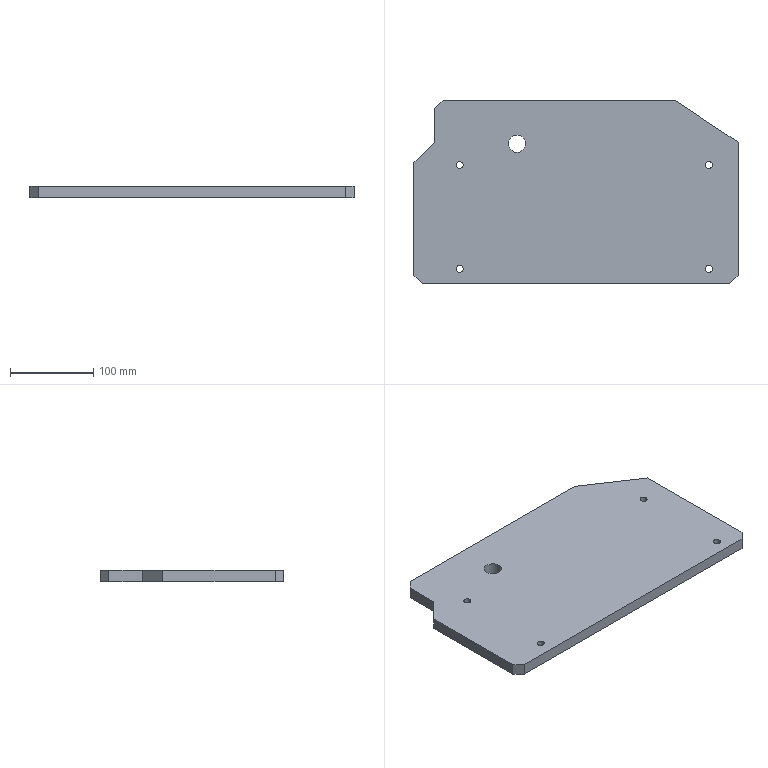Part | SolidWorks | features ICE 2, Chamfer 1, Extrusion 1, HoleWzd 1 | 1 solid | 22 faces | box 390 x 220 x 14 mm | volume 1142948 mm3 | plane 12 | cylinder 10 | commonest cylinder face diameters 8.5 x8 21 x2
STEP:
#1=CARTESIAN_POINT('',(50.75,142.5,0.));
#2=VERTEX_POINT('',#1);
#3=CARTESIAN_POINT('',(59.25,142.5,0.));
#4=VERTEX_POINT('',#3);
#5=CARTESIAN_POINT('',(55.,142.5,0.));
#6=DIRECTION('',(0.,0.,1.));
#7=DIRECTION('',(1.,0.,0.));
#8=AXIS2_PLACEMENT_3D('',#5,#6,#7);
#9=CIRCLE('',#8,4.25);
#10=EDGE_CURVE('',#2,#4,#9,.T.);
#11=ORIENTED_EDGE('',*,*,#10,.F.);
#12=CARTESIAN_POINT('',(50.75,142.5,14.));
#13=VERTEX_POINT('',#12);
#14=CARTESIAN_POINT('',(50.75,142.5,14.));
#15=DIRECTION('',(0.,0.,1.));
#16=VECTOR('',#15,1000.);
#17=LINE('',#14,#16);
#18=EDGE_CURVE('',#2,#13,#17,.T.);
#19=ORIENTED_EDGE('',*,*,#18,.T.);
#20=CARTESIAN_POINT('',(59.25,142.5,14.));
#21=VERTEX_POINT('',#20);
#22=CARTESIAN_POINT('',(55.,142.5,14.));
#23=DIRECTION('',(0.,0.,1.));
#24=DIRECTION('',(1.,0.,0.));
#25=AXIS2_PLACEMENT_3D('',#22,#23,#24);
#26=CIRCLE('',#25,4.25);
#27=EDGE_CURVE('',#13,#21,#26,.T.);
#28=ORIENTED_EDGE('',*,*,#27,.T.);
#29=CARTESIAN_POINT('',(59.25,142.5,14.));
#30=DIRECTION('',(0.,0.,1.));
#31=VECTOR('',#30,1000.);
#32=LINE('',#29,#31);
#33=EDGE_CURVE('',#4,#21,#32,.T.);
#34=ORIENTED_EDGE('',*,*,#33,.F.);
#35=EDGE_LOOP('',(#11,#19,#28,#34));
#36=FACE_OUTER_BOUND('',#35,.T.);
#37=CARTESIAN_POINT('',(55.,142.5,14.));
#38=DIRECTION('',(0.,0.,1.));
#39=DIRECTION('',(1.,0.,0.));
#40=AXIS2_PLACEMENT_3D('',#37,#38,#39);
#41=CYLINDRICAL_SURFACE('',#40,4.25);
#42=ADVANCED_FACE('',(#36),#41,.F.);
#43=CARTESIAN_POINT('',(50.75,17.5,0.));
#44=VERTEX_POINT('',#43);
#45=CARTESIAN_POINT('',(59.25,17.5,0.));
#46=VERTEX_POINT('',#45);
#47=CARTESIAN_POINT('',(55.,17.5,0.));
#48=DIRECTION('',(0.,0.,1.));
#49=DIRECTION('',(1.,0.,0.));
#50=AXIS2_PLACEMENT_3D('',#47,#48,#49);
#51=CIRCLE('',#50,4.25);
#52=EDGE_CURVE('',#44,#46,#51,.T.);
#53=ORIENTED_EDGE('',*,*,#52,.F.);
#54=CARTESIAN_POINT('',(50.75,17.5,14.));
#55=VERTEX_POINT('',#54);
#56=CARTESIAN_POINT('',(50.75,17.5,14.));
#57=DIRECTION('',(0.,0.,1.));
#58=VECTOR('',#57,1000.);
#59=LINE('',#56,#58);
#60=EDGE_CURVE('',#44,#55,#59,.T.);
#61=ORIENTED_EDGE('',*,*,#60,.T.);
#62=CARTESIAN_POINT('',(59.25,17.5,14.));
#63=VERTEX_POINT('',#62);
#64=CARTESIAN_POINT('',(55.,17.5,14.));
#65=DIRECTION('',(0.,0.,1.));
#66=DIRECTION('',(1.,0.,0.));
#67=AXIS2_PLACEMENT_3D('',#64,#65,#66);
#68=CIRCLE('',#67,4.25);
#69=EDGE_CURVE('',#55,#63,#68,.T.);
#70=ORIENTED_EDGE('',*,*,#69,.T.);
#71=CARTESIAN_POINT('',(59.25,17.5,14.));
#72=DIRECTION('',(0.,0.,1.));
#73=VECTOR('',#72,1000.);
#74=LINE('',#71,#73);
#75=EDGE_CURVE('',#46,#63,#74,.T.);
#76=ORIENTED_EDGE('',*,*,#75,.F.);
#77=EDGE_LOOP('',(#53,#61,#70,#76));
#78=FACE_OUTER_BOUND('',#77,.T.);
#79=CARTESIAN_POINT('',(55.,17.5,14.));
#80=DIRECTION('',(0.,0.,1.));
#81=DIRECTION('',(1.,0.,0.));
#82=AXIS2_PLACEMENT_3D('',#79,#80,#81);
#83=CYLINDRICAL_SURFACE('',#82,4.25);
#84=ADVANCED_FACE('',(#78),#83,.F.);
#85=CARTESIAN_POINT('',(350.75,142.5,0.));
#86=VERTEX_POINT('',#85);
#87=CARTESIAN_POINT('',(359.25,142.5,0.));
#88=VERTEX_POINT('',#87);
#89=CARTESIAN_POINT('',(355.,142.5,0.));
#90=DIRECTION('',(0.,0.,1.));
#91=DIRECTION('',(1.,0.,0.));
#92=AXIS2_PLACEMENT_3D('',#89,#90,#91);
#93=CIRCLE('',#92,4.25);
#94=EDGE_CURVE('',#86,#88,#93,.T.);
#95=ORIENTED_EDGE('',*,*,#94,.F.);
#96=CARTESIAN_POINT('',(350.75,142.5,14.));
#97=VERTEX_POINT('',#96);
#98=CARTESIAN_POINT('',(350.75,142.5,14.));
#99=DIRECTION('',(0.,0.,1.));
#100=VECTOR('',#99,1000.);
#101=LINE('',#98,#100);
#102=EDGE_CURVE('',#86,#97,#101,.T.);
#103=ORIENTED_EDGE('',*,*,#102,.T.);
#104=CARTESIAN_POINT('',(359.25,142.5,14.));
#105=VERTEX_POINT('',#104);
#106=CARTESIAN_POINT('',(355.,142.5,14.));
#107=DIRECTION('',(0.,0.,1.));
#108=DIRECTION('',(1.,0.,0.));
#109=AXIS2_PLACEMENT_3D('',#106,#107,#108);
#110=CIRCLE('',#109,4.25);
#111=EDGE_CURVE('',#97,#105,#110,.T.);
#112=ORIENTED_EDGE('',*,*,#111,.T.);
#113=CARTESIAN_POINT('',(359.25,142.5,14.));
#114=DIRECTION('',(0.,0.,1.));
#115=VECTOR('',#114,1000.);
#116=LINE('',#113,#115);
#117=EDGE_CURVE('',#88,#105,#116,.T.);
#118=ORIENTED_EDGE('',*,*,#117,.F.);
#119=EDGE_LOOP('',(#95,#103,#112,#118));
#120=FACE_OUTER_BOUND('',#119,.T.);
#121=CARTESIAN_POINT('',(355.,142.5,14.));
#122=DIRECTION('',(0.,0.,1.));
#123=DIRECTION('',(1.,0.,0.));
#124=AXIS2_PLACEMENT_3D('',#121,#122,#123);
#125=CYLINDRICAL_SURFACE('',#124,4.25);
#126=ADVANCED_FACE('',(#120),#125,.F.);
#127=CARTESIAN_POINT('',(350.75,17.5,0.));
#128=VERTEX_POINT('',#127);
#129=CARTESIAN_POINT('',(359.25,17.5,0.));
#130=VERTEX_POINT('',#129);
#131=CARTESIAN_POINT('',(355.,17.5,0.));
#132=DIRECTION('',(0.,0.,1.));
#133=DIRECTION('',(1.,0.,0.));
#134=AXIS2_PLACEMENT_3D('',#131,#132,#133);
#135=CIRCLE('',#134,4.25);
#136=EDGE_CURVE('',#128,#130,#135,.T.);
#137=ORIENTED_EDGE('',*,*,#136,.F.);
#138=CARTESIAN_POINT('',(350.75,17.5,14.));
#139=VERTEX_POINT('',#138);
#140=CARTESIAN_POINT('',(350.75,17.5,14.));
#141=DIRECTION('',(0.,0.,1.));
#142=VECTOR('',#141,1000.);
#143=LINE('',#140,#142);
#144=EDGE_CURVE('',#128,#139,#143,.T.);
#145=ORIENTED_EDGE('',*,*,#144,.T.);
#146=CARTESIAN_POINT('',(359.25,17.5,14.));
#147=VERTEX_POINT('',#146);
#148=CARTESIAN_POINT('',(355.,17.5,14.));
#149=DIRECTION('',(0.,0.,1.));
#150=DIRECTION('',(1.,0.,0.));
#151=AXIS2_PLACEMENT_3D('',#148,#149,#150);
#152=CIRCLE('',#151,4.25);
#153=EDGE_CURVE('',#139,#147,#152,.T.);
#154=ORIENTED_EDGE('',*,*,#153,.T.);
#155=CARTESIAN_POINT('',(359.25,17.5,14.));
#156=DIRECTION('',(0.,0.,1.));
#157=VECTOR('',#156,1000.);
#158=LINE('',#155,#157);
#159=EDGE_CURVE('',#130,#147,#158,.T.);
#160=ORIENTED_EDGE('',*,*,#159,.F.);
#161=EDGE_LOOP('',(#137,#145,#154,#160));
#162=FACE_OUTER_BOUND('',#161,.T.);
#163=CARTESIAN_POINT('',(355.,17.5,14.));
#164=DIRECTION('',(0.,0.,1.));
#165=DIRECTION('',(1.,0.,0.));
#166=AXIS2_PLACEMENT_3D('',#163,#164,#165);
#167=CYLINDRICAL_SURFACE('',#166,4.25);
#168=ADVANCED_FACE('',(#162),#167,.F.);
#169=CARTESIAN_POINT('',(113.5,168.,14.));
#170=VERTEX_POINT('',#169);
#171=CARTESIAN_POINT('',(134.5,168.,14.));
#172=VERTEX_POINT('',#171);
#173=CARTESIAN_POINT('',(124.,168.,14.));
#174=DIRECTION('',(0.,0.,1.));
#175=DIRECTION('',(1.,0.,0.));
#176=AXIS2_PLACEMENT_3D('',#173,#174,#175);
#177=CIRCLE('',#176,10.5);
#178=EDGE_CURVE('',#170,#172,#177,.T.);
#179=ORIENTED_EDGE('',*,*,#178,.T.);
#180=CARTESIAN_POINT('',(134.5,168.,0.));
#181=VERTEX_POINT('',#180);
#182=CARTESIAN_POINT('',(134.5,168.,14.));
#183=DIRECTION('',(0.,0.,-1.));
#184=VECTOR('',#183,1000.);
#185=LINE('',#182,#184);
#186=EDGE_CURVE('',#172,#181,#185,.T.);
#187=ORIENTED_EDGE('',*,*,#186,.T.);
#188=CARTESIAN_POINT('',(113.5,168.,0.));
#189=VERTEX_POINT('',#188);
#190=CARTESIAN_POINT('',(124.,168.,0.));
#191=DIRECTION('',(0.,0.,1.));
#192=DIRECTION('',(1.,0.,0.));
#193=AXIS2_PLACEMENT_3D('',#190,#191,#192);
#194=CIRCLE('',#193,10.5);
#195=EDGE_CURVE('',#189,#181,#194,.T.);
#196=ORIENTED_EDGE('',*,*,#195,.F.);
#197=CARTESIAN_POINT('',(113.5,168.,14.));
#198=DIRECTION('',(0.,0.,-1.));
#199=VECTOR('',#198,1000.);
#200=LINE('',#197,#199);
#201=EDGE_CURVE('',#170,#189,#200,.T.);
#202=ORIENTED_EDGE('',*,*,#201,.F.);
#203=EDGE_LOOP('',(#179,#187,#196,#202));
#204=FACE_OUTER_BOUND('',#203,.T.);
#205=CARTESIAN_POINT('',(124.,168.,14.));
#206=DIRECTION('',(0.,0.,-1.));
#207=DIRECTION('',(-1.,0.,0.));
#208=AXIS2_PLACEMENT_3D('',#205,#206,#207);
#209=CYLINDRICAL_SURFACE('',#208,10.5);
#210=ADVANCED_FACE('',(#204),#209,.F.);
#211=CARTESIAN_POINT('',(55.,142.5,14.));
#212=DIRECTION('',(0.,0.,1.));
#213=DIRECTION('',(1.,0.,0.));
#214=AXIS2_PLACEMENT_3D('',#211,#212,#213);
#215=CIRCLE('',#214,4.25);
#216=EDGE_CURVE('',#21,#13,#215,.T.);
#217=ORIENTED_EDGE('',*,*,#216,.F.);
#218=ORIENTED_EDGE('',*,*,#27,.F.);
#219=EDGE_LOOP('',(#217,#218));
#220=FACE_BOUND('',#219,.T.);
#221=CARTESIAN_POINT('',(55.,17.5,14.));
#222=DIRECTION('',(0.,0.,1.));
#223=DIRECTION('',(1.,0.,0.));
#224=AXIS2_PLACEMENT_3D('',#221,#222,#223);
#225=CIRCLE('',#224,4.25);
#226=EDGE_CURVE('',#63,#55,#225,.T.);
#227=ORIENTED_EDGE('',*,*,#226,.F.);
#228=ORIENTED_EDGE('',*,*,#69,.F.);
#229=EDGE_LOOP('',(#227,#228));
#230=FACE_BOUND('',#229,.T.);
#231=CARTESIAN_POINT('',(355.,142.5,14.));
#232=DIRECTION('',(0.,0.,1.));
#233=DIRECTION('',(1.,0.,0.));
#234=AXIS2_PLACEMENT_3D('',#231,#232,#233);
#235=CIRCLE('',#234,4.25);
#236=EDGE_CURVE('',#105,#97,#235,.T.);
#237=ORIENTED_EDGE('',*,*,#236,.F.);
#238=ORIENTED_EDGE('',*,*,#111,.F.);
#239=EDGE_LOOP('',(#237,#238));
#240=FACE_BOUND('',#239,.T.);
#241=CARTESIAN_POINT('',(25.,170.,14.));
#242=VERTEX_POINT('',#241);
#243=CARTESIAN_POINT('',(0.,145.,14.));
#244=VERTEX_POINT('',#243);
#245=CARTESIAN_POINT('',(-72.5,72.5,14.));
#246=DIRECTION('',(-0.7071,-0.7071,0.));
#247=VECTOR('',#246,1000.);
#248=LINE('',#245,#247);
#249=EDGE_CURVE('',#242,#244,#248,.T.);
#250=ORIENTED_EDGE('',*,*,#249,.T.);
#251=CARTESIAN_POINT('',(0.,10.,14.));
#252=VERTEX_POINT('',#251);
#253=CARTESIAN_POINT('',(0.,0.,14.));
#254=DIRECTION('',(0.,-1.,0.));
#255=VECTOR('',#254,1000.);
#256=LINE('',#253,#255);
#257=EDGE_CURVE('',#244,#252,#256,.T.);
#258=ORIENTED_EDGE('',*,*,#257,.T.);
#259=CARTESIAN_POINT('',(10.,0.,14.));
#260=VERTEX_POINT('',#259);
#261=CARTESIAN_POINT('',(10.,0.,14.));
#262=DIRECTION('',(0.7071,-0.7071,0.));
#263=VECTOR('',#262,1000.);
#264=LINE('',#261,#263);
#265=EDGE_CURVE('',#252,#260,#264,.T.);
#266=ORIENTED_EDGE('',*,*,#265,.T.);
#267=CARTESIAN_POINT('',(380.,0.,14.));
#268=VERTEX_POINT('',#267);
#269=CARTESIAN_POINT('',(390.,0.,14.));
#270=DIRECTION('',(1.,0.,0.));
#271=VECTOR('',#270,1000.);
#272=LINE('',#269,#271);
#273=EDGE_CURVE('',#260,#268,#272,.T.);
#274=ORIENTED_EDGE('',*,*,#273,.T.);
#275=CARTESIAN_POINT('',(390.,10.,14.));
#276=VERTEX_POINT('',#275);
#277=CARTESIAN_POINT('',(390.,10.,14.));
#278=DIRECTION('',(0.7071,0.7071,0.));
#279=VECTOR('',#278,1000.);
#280=LINE('',#277,#279);
#281=EDGE_CURVE('',#268,#276,#280,.T.);
#282=ORIENTED_EDGE('',*,*,#281,.T.);
#283=CARTESIAN_POINT('',(390.,170.,14.));
#284=VERTEX_POINT('',#283);
#285=CARTESIAN_POINT('',(390.,170.,14.));
#286=DIRECTION('',(0.,1.,0.));
#287=VECTOR('',#286,1000.);
#288=LINE('',#285,#287);
#289=EDGE_CURVE('',#276,#284,#288,.T.);
#290=ORIENTED_EDGE('',*,*,#289,.T.);
#291=CARTESIAN_POINT('',(315.,220.,14.));
#292=VERTEX_POINT('',#291);
#293=CARTESIAN_POINT('',(315.,220.,14.));
#294=DIRECTION('',(-0.8321,0.5547,0.));
#295=VECTOR('',#294,1000.);
#296=LINE('',#293,#295);
#297=EDGE_CURVE('',#284,#292,#296,.T.);
#298=ORIENTED_EDGE('',*,*,#297,.T.);
#299=CARTESIAN_POINT('',(35.,220.,14.));
#300=VERTEX_POINT('',#299);
#301=CARTESIAN_POINT('',(0.,220.,14.));
#302=DIRECTION('',(-1.,0.,0.));
#303=VECTOR('',#302,1000.);
#304=LINE('',#301,#303);
#305=EDGE_CURVE('',#292,#300,#304,.T.);
#306=ORIENTED_EDGE('',*,*,#305,.T.);
#307=CARTESIAN_POINT('',(25.,210.,14.));
#308=VERTEX_POINT('',#307);
#309=CARTESIAN_POINT('',(35.,220.,14.));
#310=DIRECTION('',(-0.7071,-0.7071,0.));
#311=VECTOR('',#310,1000.);
#312=LINE('',#309,#311);
#313=EDGE_CURVE('',#300,#308,#312,.T.);
#314=ORIENTED_EDGE('',*,*,#313,.T.);
#315=CARTESIAN_POINT('',(25.,220.,14.));
#316=DIRECTION('',(0.,1.,0.));
#317=VECTOR('',#316,1000.);
#318=LINE('',#315,#317);
#319=EDGE_CURVE('',#242,#308,#318,.T.);
#320=ORIENTED_EDGE('',*,*,#319,.F.);
#321=EDGE_LOOP('',(#250,#258,#266,#274,#282,#290,#298,#306,#314,#320));
#322=FACE_OUTER_BOUND('',#321,.T.);
#323=ORIENTED_EDGE('',*,*,#178,.F.);
#324=CARTESIAN_POINT('',(124.,168.,14.));
#325=DIRECTION('',(0.,0.,1.));
#326=DIRECTION('',(1.,0.,0.));
#327=AXIS2_PLACEMENT_3D('',#324,#325,#326);
#328=CIRCLE('',#327,10.5);
#329=EDGE_CURVE('',#172,#170,#328,.T.);
#330=ORIENTED_EDGE('',*,*,#329,.F.);
#331=EDGE_LOOP('',(#323,#330));
#332=FACE_BOUND('',#331,.T.);
#333=CARTESIAN_POINT('',(355.,17.5,14.));
#334=DIRECTION('',(0.,0.,1.));
#335=DIRECTION('',(1.,0.,0.));
#336=AXIS2_PLACEMENT_3D('',#333,#334,#335);
#337=CIRCLE('',#336,4.25);
#338=EDGE_CURVE('',#147,#139,#337,.T.);
#339=ORIENTED_EDGE('',*,*,#338,.F.);
#340=ORIENTED_EDGE('',*,*,#153,.F.);
#341=EDGE_LOOP('',(#339,#340));
#342=FACE_BOUND('',#341,.T.);
#343=CARTESIAN_POINT('',(0.,0.,14.));
#344=DIRECTION('',(0.,0.,-1.));
#345=DIRECTION('',(-1.,0.,0.));
#346=AXIS2_PLACEMENT_3D('',#343,#344,#345);
#347=PLANE('',#346);
#348=ADVANCED_FACE('',(#220,#230,#240,#322,#332,#342),#347,.F.);
#349=CARTESIAN_POINT('',(0.,145.,0.));
#350=VERTEX_POINT('',#349);
#351=CARTESIAN_POINT('',(0.,10.,0.));
#352=VERTEX_POINT('',#351);
#353=CARTESIAN_POINT('',(0.,0.,0.));
#354=DIRECTION('',(0.,-1.,0.));
#355=VECTOR('',#354,1000.);
#356=LINE('',#353,#355);
#357=EDGE_CURVE('',#350,#352,#356,.T.);
#358=ORIENTED_EDGE('',*,*,#357,.F.);
#359=CARTESIAN_POINT('',(25.,170.,0.));
#360=VERTEX_POINT('',#359);
#361=CARTESIAN_POINT('',(25.,170.,0.));
#362=DIRECTION('',(0.7071,0.7071,0.));
#363=VECTOR('',#362,1000.);
#364=LINE('',#361,#363);
#365=EDGE_CURVE('',#350,#360,#364,.T.);
#366=ORIENTED_EDGE('',*,*,#365,.T.);
#367=CARTESIAN_POINT('',(25.,210.,0.));
#368=VERTEX_POINT('',#367);
#369=CARTESIAN_POINT('',(25.,220.,0.));
#370=DIRECTION('',(0.,1.,0.));
#371=VECTOR('',#370,1000.);
#372=LINE('',#369,#371);
#373=EDGE_CURVE('',#360,#368,#372,.T.);
#374=ORIENTED_EDGE('',*,*,#373,.T.);
#375=CARTESIAN_POINT('',(35.,220.,0.));
#376=VERTEX_POINT('',#375);
#377=CARTESIAN_POINT('',(-92.5,92.5,0.));
#378=DIRECTION('',(0.7071,0.7071,0.));
#379=VECTOR('',#378,1000.);
#380=LINE('',#377,#379);
#381=EDGE_CURVE('',#368,#376,#380,.T.);
#382=ORIENTED_EDGE('',*,*,#381,.T.);
#383=CARTESIAN_POINT('',(315.,220.,0.));
#384=VERTEX_POINT('',#383);
#385=CARTESIAN_POINT('',(0.,220.,0.));
#386=DIRECTION('',(-1.,0.,0.));
#387=VECTOR('',#386,1000.);
#388=LINE('',#385,#387);
#389=EDGE_CURVE('',#384,#376,#388,.T.);
#390=ORIENTED_EDGE('',*,*,#389,.F.);
#391=CARTESIAN_POINT('',(390.,170.,0.));
#392=VERTEX_POINT('',#391);
#393=CARTESIAN_POINT('',(315.,220.,0.));
#394=DIRECTION('',(-0.8321,0.5547,0.));
#395=VECTOR('',#394,1000.);
#396=LINE('',#393,#395);
#397=EDGE_CURVE('',#392,#384,#396,.T.);
#398=ORIENTED_EDGE('',*,*,#397,.F.);
#399=CARTESIAN_POINT('',(390.,10.,0.));
#400=VERTEX_POINT('',#399);
#401=CARTESIAN_POINT('',(390.,170.,0.));
#402=DIRECTION('',(0.,1.,0.));
#403=VECTOR('',#402,1000.);
#404=LINE('',#401,#403);
#405=EDGE_CURVE('',#400,#392,#404,.T.);
#406=ORIENTED_EDGE('',*,*,#405,.F.);
#407=CARTESIAN_POINT('',(380.,0.,0.));
#408=VERTEX_POINT('',#407);
#409=CARTESIAN_POINT('',(190.,-190.,0.));
#410=DIRECTION('',(-0.7071,-0.7071,0.));
#411=VECTOR('',#410,1000.);
#412=LINE('',#409,#411);
#413=EDGE_CURVE('',#400,#408,#412,.T.);
#414=ORIENTED_EDGE('',*,*,#413,.T.);
#415=CARTESIAN_POINT('',(10.,0.,0.));
#416=VERTEX_POINT('',#415);
#417=CARTESIAN_POINT('',(390.,0.,0.));
#418=DIRECTION('',(1.,0.,0.));
#419=VECTOR('',#418,1000.);
#420=LINE('',#417,#419);
#421=EDGE_CURVE('',#416,#408,#420,.T.);
#422=ORIENTED_EDGE('',*,*,#421,.F.);
#423=CARTESIAN_POINT('',(5.,5.,0.));
#424=DIRECTION('',(-0.7071,0.7071,0.));
#425=VECTOR('',#424,1000.);
#426=LINE('',#423,#425);
#427=EDGE_CURVE('',#416,#352,#426,.T.);
#428=ORIENTED_EDGE('',*,*,#427,.T.);
#429=EDGE_LOOP('',(#358,#366,#374,#382,#390,#398,#406,#414,#422,#428));
#430=FACE_OUTER_BOUND('',#429,.T.);
#431=CARTESIAN_POINT('',(55.,142.5,0.));
#432=DIRECTION('',(0.,0.,1.));
#433=DIRECTION('',(1.,0.,0.));
#434=AXIS2_PLACEMENT_3D('',#431,#432,#433);
#435=CIRCLE('',#434,4.25);
#436=EDGE_CURVE('',#4,#2,#435,.T.);
#437=ORIENTED_EDGE('',*,*,#436,.T.);
#438=ORIENTED_EDGE('',*,*,#10,.T.);
#439=EDGE_LOOP('',(#437,#438));
#440=FACE_BOUND('',#439,.T.);
#441=CARTESIAN_POINT('',(55.,17.5,0.));
#442=DIRECTION('',(0.,0.,1.));
#443=DIRECTION('',(1.,0.,0.));
#444=AXIS2_PLACEMENT_3D('',#441,#442,#443);
#445=CIRCLE('',#444,4.25);
#446=EDGE_CURVE('',#46,#44,#445,.T.);
#447=ORIENTED_EDGE('',*,*,#446,.T.);
#448=ORIENTED_EDGE('',*,*,#52,.T.);
#449=EDGE_LOOP('',(#447,#448));
#450=FACE_BOUND('',#449,.T.);
#451=CARTESIAN_POINT('',(355.,142.5,0.));
#452=DIRECTION('',(0.,0.,1.));
#453=DIRECTION('',(1.,0.,0.));
#454=AXIS2_PLACEMENT_3D('',#451,#452,#453);
#455=CIRCLE('',#454,4.25);
#456=EDGE_CURVE('',#88,#86,#455,.T.);
#457=ORIENTED_EDGE('',*,*,#456,.T.);
#458=ORIENTED_EDGE('',*,*,#94,.T.);
#459=EDGE_LOOP('',(#457,#458));
#460=FACE_BOUND('',#459,.T.);
#461=ORIENTED_EDGE('',*,*,#195,.T.);
#462=CARTESIAN_POINT('',(124.,168.,0.));
#463=DIRECTION('',(0.,0.,1.));
#464=DIRECTION('',(1.,0.,0.));
#465=AXIS2_PLACEMENT_3D('',#462,#463,#464);
#466=CIRCLE('',#465,10.5);
#467=EDGE_CURVE('',#181,#189,#466,.T.);
#468=ORIENTED_EDGE('',*,*,#467,.T.);
#469=EDGE_LOOP('',(#461,#468));
#470=FACE_BOUND('',#469,.T.);
#471=CARTESIAN_POINT('',(355.,17.5,0.));
#472=DIRECTION('',(0.,0.,1.));
#473=DIRECTION('',(1.,0.,0.));
#474=AXIS2_PLACEMENT_3D('',#471,#472,#473);
#475=CIRCLE('',#474,4.25);
#476=EDGE_CURVE('',#130,#128,#475,.T.);
#477=ORIENTED_EDGE('',*,*,#476,.T.);
#478=ORIENTED_EDGE('',*,*,#136,.T.);
#479=EDGE_LOOP('',(#477,#478));
#480=FACE_BOUND('',#479,.T.);
#481=CARTESIAN_POINT('',(0.,0.,0.));
#482=DIRECTION('',(0.,0.,-1.));
#483=DIRECTION('',(-1.,0.,0.));
#484=AXIS2_PLACEMENT_3D('',#481,#482,#483);
#485=PLANE('',#484);
#486=ADVANCED_FACE('',(#430,#440,#450,#460,#470,#480),#485,.T.);
#487=ORIENTED_EDGE('',*,*,#257,.F.);
#488=CARTESIAN_POINT('',(0.,145.,0.));
#489=DIRECTION('',(0.,0.,1.));
#490=VECTOR('',#489,1000.);
#491=LINE('',#488,#490);
#492=EDGE_CURVE('',#350,#244,#491,.T.);
#493=ORIENTED_EDGE('',*,*,#492,.F.);
#494=ORIENTED_EDGE('',*,*,#357,.T.);
#495=CARTESIAN_POINT('',(0.,10.,14.));
#496=DIRECTION('',(0.,0.,1.));
#497=VECTOR('',#496,1000.);
#498=LINE('',#495,#497);
#499=EDGE_CURVE('',#352,#252,#498,.T.);
#500=ORIENTED_EDGE('',*,*,#499,.T.);
#501=EDGE_LOOP('',(#487,#493,#494,#500));
#502=FACE_OUTER_BOUND('',#501,.T.);
#503=CARTESIAN_POINT('',(0.,0.,14.));
#504=DIRECTION('',(1.,0.,0.));
#505=DIRECTION('',(0.,0.,-1.));
#506=AXIS2_PLACEMENT_3D('',#503,#504,#505);
#507=PLANE('',#506);
#508=ADVANCED_FACE('',(#502),#507,.F.);
#509=ORIENTED_EDGE('',*,*,#421,.T.);
#510=CARTESIAN_POINT('',(380.,0.,14.));
#511=DIRECTION('',(0.,0.,1.));
#512=VECTOR('',#511,1000.);
#513=LINE('',#510,#512);
#514=EDGE_CURVE('',#408,#268,#513,.T.);
#515=ORIENTED_EDGE('',*,*,#514,.T.);
#516=ORIENTED_EDGE('',*,*,#273,.F.);
#517=CARTESIAN_POINT('',(10.,0.,14.));
#518=DIRECTION('',(0.,0.,-1.));
#519=VECTOR('',#518,1000.);
#520=LINE('',#517,#519);
#521=EDGE_CURVE('',#260,#416,#520,.T.);
#522=ORIENTED_EDGE('',*,*,#521,.T.);
#523=EDGE_LOOP('',(#509,#515,#516,#522));
#524=FACE_OUTER_BOUND('',#523,.T.);
#525=CARTESIAN_POINT('',(390.,0.,14.));
#526=DIRECTION('',(0.,1.,0.));
#527=DIRECTION('',(-1.,0.,0.));
#528=AXIS2_PLACEMENT_3D('',#525,#526,#527);
#529=PLANE('',#528);
#530=ADVANCED_FACE('',(#524),#529,.F.);
#531=ORIENTED_EDGE('',*,*,#289,.F.);
#532=CARTESIAN_POINT('',(390.,10.,14.));
#533=DIRECTION('',(0.,0.,-1.));
#534=VECTOR('',#533,1000.);
#535=LINE('',#532,#534);
#536=EDGE_CURVE('',#276,#400,#535,.T.);
#537=ORIENTED_EDGE('',*,*,#536,.T.);
#538=ORIENTED_EDGE('',*,*,#405,.T.);
#539=CARTESIAN_POINT('',(390.,170.,14.));
#540=DIRECTION('',(0.,0.,-1.));
#541=VECTOR('',#540,1000.);
#542=LINE('',#539,#541);
#543=EDGE_CURVE('',#284,#392,#542,.T.);
#544=ORIENTED_EDGE('',*,*,#543,.F.);
#545=EDGE_LOOP('',(#531,#537,#538,#544));
#546=FACE_OUTER_BOUND('',#545,.T.);
#547=CARTESIAN_POINT('',(390.,170.,14.));
#548=DIRECTION('',(-1.,0.,0.));
#549=DIRECTION('',(0.,0.,1.));
#550=AXIS2_PLACEMENT_3D('',#547,#548,#549);
#551=PLANE('',#550);
#552=ADVANCED_FACE('',(#546),#551,.F.);
#553=ORIENTED_EDGE('',*,*,#397,.T.);
#554=CARTESIAN_POINT('',(315.,220.,14.));
#555=DIRECTION('',(0.,0.,-1.));
#556=VECTOR('',#555,1000.);
#557=LINE('',#554,#556);
#558=EDGE_CURVE('',#292,#384,#557,.T.);
#559=ORIENTED_EDGE('',*,*,#558,.F.);
#560=ORIENTED_EDGE('',*,*,#297,.F.);
#561=ORIENTED_EDGE('',*,*,#543,.T.);
#562=EDGE_LOOP('',(#553,#559,#560,#561));
#563=FACE_OUTER_BOUND('',#562,.T.);
#564=CARTESIAN_POINT('',(315.,220.,14.));
#565=DIRECTION('',(-0.5547,-0.8321,0.));
#566=DIRECTION('',(0.8321,-0.5547,0.));
#567=AXIS2_PLACEMENT_3D('',#564,#565,#566);
#568=PLANE('',#567);
#569=ADVANCED_FACE('',(#563),#568,.F.);
#570=ORIENTED_EDGE('',*,*,#389,.T.);
#571=CARTESIAN_POINT('',(35.,220.,14.));
#572=DIRECTION('',(0.,0.,1.));
#573=VECTOR('',#572,1000.);
#574=LINE('',#571,#573);
#575=EDGE_CURVE('',#376,#300,#574,.T.);
#576=ORIENTED_EDGE('',*,*,#575,.T.);
#577=ORIENTED_EDGE('',*,*,#305,.F.);
#578=ORIENTED_EDGE('',*,*,#558,.T.);
#579=EDGE_LOOP('',(#570,#576,#577,#578));
#580=FACE_OUTER_BOUND('',#579,.T.);
#581=CARTESIAN_POINT('',(0.,220.,14.));
#582=DIRECTION('',(0.,-1.,0.));
#583=DIRECTION('',(0.,0.,-1.));
#584=AXIS2_PLACEMENT_3D('',#581,#582,#583);
#585=PLANE('',#584);
#586=ADVANCED_FACE('',(#580),#585,.F.);
#587=ORIENTED_EDGE('',*,*,#186,.F.);
#588=ORIENTED_EDGE('',*,*,#329,.T.);
#589=ORIENTED_EDGE('',*,*,#201,.T.);
#590=ORIENTED_EDGE('',*,*,#467,.F.);
#591=EDGE_LOOP('',(#587,#588,#589,#590));
#592=FACE_OUTER_BOUND('',#591,.T.);
#593=CARTESIAN_POINT('',(124.,168.,14.));
#594=DIRECTION('',(0.,0.,-1.));
#595=DIRECTION('',(-1.,0.,0.));
#596=AXIS2_PLACEMENT_3D('',#593,#594,#595);
#597=CYLINDRICAL_SURFACE('',#596,10.5);
#598=ADVANCED_FACE('',(#592),#597,.F.);
#599=ORIENTED_EDGE('',*,*,#144,.F.);
#600=ORIENTED_EDGE('',*,*,#476,.F.);
#601=ORIENTED_EDGE('',*,*,#159,.T.);
#602=ORIENTED_EDGE('',*,*,#338,.T.);
#603=EDGE_LOOP('',(#599,#600,#601,#602));
#604=FACE_OUTER_BOUND('',#603,.T.);
#605=CARTESIAN_POINT('',(355.,17.5,14.));
#606=DIRECTION('',(0.,0.,1.));
#607=DIRECTION('',(1.,0.,0.));
#608=AXIS2_PLACEMENT_3D('',#605,#606,#607);
#609=CYLINDRICAL_SURFACE('',#608,4.25);
#610=ADVANCED_FACE('',(#604),#609,.F.);
#611=ORIENTED_EDGE('',*,*,#102,.F.);
#612=ORIENTED_EDGE('',*,*,#456,.F.);
#613=ORIENTED_EDGE('',*,*,#117,.T.);
#614=ORIENTED_EDGE('',*,*,#236,.T.);
#615=EDGE_LOOP('',(#611,#612,#613,#614));
#616=FACE_OUTER_BOUND('',#615,.T.);
#617=CARTESIAN_POINT('',(355.,142.5,14.));
#618=DIRECTION('',(0.,0.,1.));
#619=DIRECTION('',(1.,0.,0.));
#620=AXIS2_PLACEMENT_3D('',#617,#618,#619);
#621=CYLINDRICAL_SURFACE('',#620,4.25);
#622=ADVANCED_FACE('',(#616),#621,.F.);
#623=ORIENTED_EDGE('',*,*,#60,.F.);
#624=ORIENTED_EDGE('',*,*,#446,.F.);
#625=ORIENTED_EDGE('',*,*,#75,.T.);
#626=ORIENTED_EDGE('',*,*,#226,.T.);
#627=EDGE_LOOP('',(#623,#624,#625,#626));
#628=FACE_OUTER_BOUND('',#627,.T.);
#629=CARTESIAN_POINT('',(55.,17.5,14.));
#630=DIRECTION('',(0.,0.,1.));
#631=DIRECTION('',(1.,0.,0.));
#632=AXIS2_PLACEMENT_3D('',#629,#630,#631);
#633=CYLINDRICAL_SURFACE('',#632,4.25);
#634=ADVANCED_FACE('',(#628),#633,.F.);
#635=ORIENTED_EDGE('',*,*,#18,.F.);
#636=ORIENTED_EDGE('',*,*,#436,.F.);
#637=ORIENTED_EDGE('',*,*,#33,.T.);
#638=ORIENTED_EDGE('',*,*,#216,.T.);
#639=EDGE_LOOP('',(#635,#636,#637,#638));
#640=FACE_OUTER_BOUND('',#639,.T.);
#641=CARTESIAN_POINT('',(55.,142.5,14.));
#642=DIRECTION('',(0.,0.,1.));
#643=DIRECTION('',(1.,0.,0.));
#644=AXIS2_PLACEMENT_3D('',#641,#642,#643);
#645=CYLINDRICAL_SURFACE('',#644,4.25);
#646=ADVANCED_FACE('',(#640),#645,.F.);
#647=ORIENTED_EDGE('',*,*,#319,.T.);
#648=CARTESIAN_POINT('',(25.,210.,0.));
#649=DIRECTION('',(0.,0.,-1.));
#650=VECTOR('',#649,1000.);
#651=LINE('',#648,#650);
#652=EDGE_CURVE('',#308,#368,#651,.T.);
#653=ORIENTED_EDGE('',*,*,#652,.T.);
#654=ORIENTED_EDGE('',*,*,#373,.F.);
#655=CARTESIAN_POINT('',(25.,170.,14.));
#656=DIRECTION('',(0.,0.,1.));
#657=VECTOR('',#656,1000.);
#658=LINE('',#655,#657);
#659=EDGE_CURVE('',#360,#242,#658,.T.);
#660=ORIENTED_EDGE('',*,*,#659,.T.);
#661=EDGE_LOOP('',(#647,#653,#654,#660));
#662=FACE_OUTER_BOUND('',#661,.T.);
#663=CARTESIAN_POINT('',(25.,220.,0.));
#664=DIRECTION('',(1.,0.,0.));
#665=DIRECTION('',(0.,1.,0.));
#666=AXIS2_PLACEMENT_3D('',#663,#664,#665);
#667=PLANE('',#666);
#668=ADVANCED_FACE('',(#662),#667,.F.);
#669=ORIENTED_EDGE('',*,*,#381,.F.);
#670=ORIENTED_EDGE('',*,*,#652,.F.);
#671=ORIENTED_EDGE('',*,*,#313,.F.);
#672=ORIENTED_EDGE('',*,*,#575,.F.);
#673=EDGE_LOOP('',(#669,#670,#671,#672));
#674=FACE_OUTER_BOUND('',#673,.T.);
#675=CARTESIAN_POINT('',(35.,220.,14.));
#676=DIRECTION('',(0.7071,-0.7071,0.));
#677=DIRECTION('',(0.,0.,1.));
#678=AXIS2_PLACEMENT_3D('',#675,#676,#677);
#679=PLANE('',#678);
#680=ADVANCED_FACE('',(#674),#679,.F.);
#681=ORIENTED_EDGE('',*,*,#365,.F.);
#682=ORIENTED_EDGE('',*,*,#492,.T.);
#683=ORIENTED_EDGE('',*,*,#249,.F.);
#684=ORIENTED_EDGE('',*,*,#659,.F.);
#685=EDGE_LOOP('',(#681,#682,#683,#684));
#686=FACE_OUTER_BOUND('',#685,.T.);
#687=CARTESIAN_POINT('',(25.,170.,0.));
#688=DIRECTION('',(-0.7071,0.7071,0.));
#689=DIRECTION('',(0.,0.,-1.));
#690=AXIS2_PLACEMENT_3D('',#687,#688,#689);
#691=PLANE('',#690);
#692=ADVANCED_FACE('',(#686),#691,.T.);
#693=ORIENTED_EDGE('',*,*,#281,.F.);
#694=ORIENTED_EDGE('',*,*,#514,.F.);
#695=ORIENTED_EDGE('',*,*,#413,.F.);
#696=ORIENTED_EDGE('',*,*,#536,.F.);
#697=EDGE_LOOP('',(#693,#694,#695,#696));
#698=FACE_OUTER_BOUND('',#697,.T.);
#699=CARTESIAN_POINT('',(390.,10.,14.));
#700=DIRECTION('',(-0.7071,0.7071,0.));
#701=DIRECTION('',(0.,0.,-1.));
#702=AXIS2_PLACEMENT_3D('',#699,#700,#701);
#703=PLANE('',#702);
#704=ADVANCED_FACE('',(#698),#703,.F.);
#705=ORIENTED_EDGE('',*,*,#265,.F.);
#706=ORIENTED_EDGE('',*,*,#499,.F.);
#707=ORIENTED_EDGE('',*,*,#427,.F.);
#708=ORIENTED_EDGE('',*,*,#521,.F.);
#709=EDGE_LOOP('',(#705,#706,#707,#708));
#710=FACE_OUTER_BOUND('',#709,.T.);
#711=CARTESIAN_POINT('',(10.,0.,14.));
#712=DIRECTION('',(0.7071,0.7071,0.));
#713=DIRECTION('',(0.,0.,-1.));
#714=AXIS2_PLACEMENT_3D('',#711,#712,#713);
#715=PLANE('',#714);
#716=ADVANCED_FACE('',(#710),#715,.F.);
#717=CLOSED_SHELL('',(#42,#84,#126,#168,#210,#348,#486,#508,#530,#552,#569,#586,#598,#610,#622,#634,#646,#668,#680,#692,#704,#716));
#718=MANIFOLD_SOLID_BREP('',#717);
#719=CARTESIAN_POINT('',(0.,0.,0.));
#720=DIRECTION('',(0.,0.,1.));
#721=DIRECTION('',(1.,0.,0.));
#722=AXIS2_PLACEMENT_3D('',#719,#720,#721);
#723=(LENGTH_UNIT()NAMED_UNIT(*)SI_UNIT(.MILLI.,.METRE.));
#724=UNCERTAINTY_MEASURE_WITH_UNIT(LENGTH_MEASURE(0.00001),#723,'','');
#725=(NAMED_UNIT(*)PLANE_ANGLE_UNIT()SI_UNIT($,.RADIAN.));
#726=(NAMED_UNIT(*)SI_UNIT($,.STERADIAN.)SOLID_ANGLE_UNIT());
#727=(GEOMETRIC_REPRESENTATION_CONTEXT(3)GLOBAL_UNCERTAINTY_ASSIGNED_CONTEXT((#724))GLOBAL_UNIT_ASSIGNED_CONTEXT((#723,#725,#726))REPRESENTATION_CONTEXT('',''));
#728=ADVANCED_BREP_SHAPE_REPRESENTATION('',(#718,#722),#727);